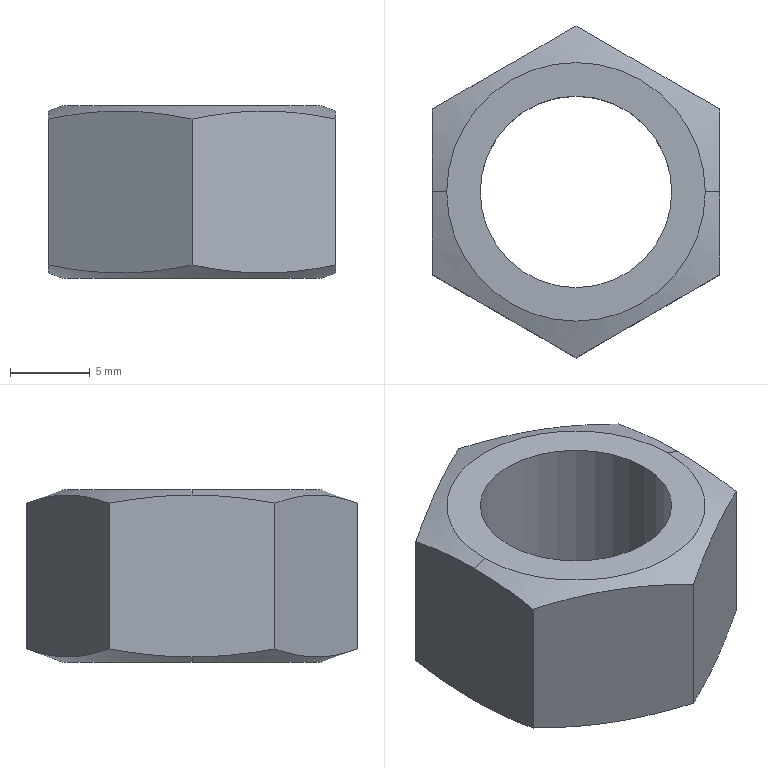Part | SolidWorks | features Extrusion 1, ICE 1, MirrorPattern 1, RefAxis 1, RevCut 1 | 1 solid | 14 faces | box 18 x 20.785 x 10.8 mm | volume 1768 mm3 | plane 8 | cone 4 | cylinder 2 | commonest cylinder face diameters 12 x2
STEP:
#1=CARTESIAN_POINT('',(-6.,0.,0.));
#2=VERTEX_POINT('',#1);
#3=CARTESIAN_POINT('',(6.,0.,0.));
#4=VERTEX_POINT('',#3);
#5=CARTESIAN_POINT('',(0.,0.,0.));
#6=DIRECTION('',(0.,0.,1.));
#7=DIRECTION('',(1.,0.,0.));
#8=AXIS2_PLACEMENT_3D('',#5,#6,#7);
#9=CIRCLE('',#8,6.);
#10=EDGE_CURVE('',#2,#4,#9,.T.);
#11=ORIENTED_EDGE('',*,*,#10,.F.);
#12=CARTESIAN_POINT('',(-6.,0.,10.8));
#13=VERTEX_POINT('',#12);
#14=CARTESIAN_POINT('',(-6.,0.,0.));
#15=DIRECTION('',(0.,0.,1.));
#16=VECTOR('',#15,1000.);
#17=LINE('',#14,#16);
#18=EDGE_CURVE('',#2,#13,#17,.T.);
#19=ORIENTED_EDGE('',*,*,#18,.T.);
#20=CARTESIAN_POINT('',(6.,0.,10.8));
#21=VERTEX_POINT('',#20);
#22=CARTESIAN_POINT('',(0.,0.,10.8));
#23=DIRECTION('',(0.,0.,1.));
#24=DIRECTION('',(1.,0.,0.));
#25=AXIS2_PLACEMENT_3D('',#22,#23,#24);
#26=CIRCLE('',#25,6.);
#27=EDGE_CURVE('',#13,#21,#26,.T.);
#28=ORIENTED_EDGE('',*,*,#27,.T.);
#29=CARTESIAN_POINT('',(6.,0.,0.));
#30=DIRECTION('',(0.,0.,1.));
#31=VECTOR('',#30,1000.);
#32=LINE('',#29,#31);
#33=EDGE_CURVE('',#4,#21,#32,.T.);
#34=ORIENTED_EDGE('',*,*,#33,.F.);
#35=EDGE_LOOP('',(#11,#19,#28,#34));
#36=FACE_OUTER_BOUND('',#35,.T.);
#37=CARTESIAN_POINT('',(0.,0.,0.));
#38=DIRECTION('',(0.,0.,1.));
#39=DIRECTION('',(1.,0.,0.));
#40=AXIS2_PLACEMENT_3D('',#37,#38,#39);
#41=CYLINDRICAL_SURFACE('',#40,6.);
#42=ADVANCED_FACE('',(#36),#41,.F.);
#43=CARTESIAN_POINT('',(-8.1,0.,0.));
#44=VERTEX_POINT('',#43);
#45=CARTESIAN_POINT('',(8.1,0.,0.));
#46=VERTEX_POINT('',#45);
#47=CARTESIAN_POINT('',(0.,0.,0.));
#48=DIRECTION('',(0.,0.,1.));
#49=DIRECTION('',(1.,0.,0.));
#50=AXIS2_PLACEMENT_3D('',#47,#48,#49);
#51=CIRCLE('',#50,8.1);
#52=EDGE_CURVE('',#44,#46,#51,.T.);
#53=ORIENTED_EDGE('',*,*,#52,.T.);
#54=CARTESIAN_POINT('',(9.,0.,0.3276));
#55=VERTEX_POINT('',#54);
#56=CARTESIAN_POINT('',(10.392,0.,0.8343));
#57=DIRECTION('',(0.9397,0.,0.342));
#58=VECTOR('',#57,1000.);
#59=LINE('',#56,#58);
#60=EDGE_CURVE('',#46,#55,#59,.T.);
#61=ORIENTED_EDGE('',*,*,#60,.T.);
#62=CARTESIAN_POINT('',(9.,-5.196,0.8343));
#63=VERTEX_POINT('',#62);
#64=CARTESIAN_POINT('',(9.,-5.196,0.8343));
#65=CARTESIAN_POINT('',(9.,-4.336,0.6778));
#66=CARTESIAN_POINT('',(9.,-3.466,0.549));
#67=CARTESIAN_POINT('',(9.,-1.732,0.3738));
#68=CARTESIAN_POINT('',(9.,-0.8653,0.3276));
#69=CARTESIAN_POINT('',(9.,0.,0.3276));
#70=B_SPLINE_CURVE_WITH_KNOTS('',3,(#64,#65,#66,#67,#68,#69),.UNSPECIFIED.,.F.,.F.,(4,2,4),(0.008807,0.01143,0.01404),.UNSPECIFIED.);
#71=EDGE_CURVE('',#63,#55,#70,.T.);
#72=ORIENTED_EDGE('',*,*,#71,.F.);
#73=CARTESIAN_POINT('',(0.,-10.392,0.8343));
#74=VERTEX_POINT('',#73);
#75=CARTESIAN_POINT('',(0.,-10.392,0.8343));
#76=CARTESIAN_POINT('',(0.75,-9.959,0.6767));
#77=CARTESIAN_POINT('',(1.5,-9.526,0.5488));
#78=CARTESIAN_POINT('',(3.,-8.66,0.3739));
#79=CARTESIAN_POINT('',(4.5,-7.794,0.2812));
#80=CARTESIAN_POINT('',(6.,-6.928,0.3739));
#81=CARTESIAN_POINT('',(7.5,-6.062,0.5488));
#82=CARTESIAN_POINT('',(8.25,-5.629,0.6767));
#83=CARTESIAN_POINT('',(9.,-5.196,0.8343));
#84=B_SPLINE_CURVE_WITH_KNOTS('',3,(#75,#76,#77,#78,#79,#80,#81,#82,#83),.UNSPECIFIED.,.F.,.F.,(4,2,1,2,4),(0.000000231,0.002598,0.005196,0.007794,0.01039),.UNSPECIFIED.);
#85=EDGE_CURVE('',#74,#63,#84,.T.);
#86=ORIENTED_EDGE('',*,*,#85,.F.);
#87=CARTESIAN_POINT('',(-9.,-5.196,0.8343));
#88=VERTEX_POINT('',#87);
#89=CARTESIAN_POINT('',(-9.,-5.196,0.8343));
#90=CARTESIAN_POINT('',(-8.25,-5.629,0.6767));
#91=CARTESIAN_POINT('',(-7.5,-6.062,0.5488));
#92=CARTESIAN_POINT('',(-6.,-6.928,0.3739));
#93=CARTESIAN_POINT('',(-4.5,-7.794,0.2812));
#94=CARTESIAN_POINT('',(-3.,-8.66,0.3739));
#95=CARTESIAN_POINT('',(-1.5,-9.526,0.5488));
#96=CARTESIAN_POINT('',(-0.75,-9.959,0.6767));
#97=CARTESIAN_POINT('',(0.,-10.392,0.8343));
#98=B_SPLINE_CURVE_WITH_KNOTS('',3,(#89,#90,#91,#92,#93,#94,#95,#96,#97),.UNSPECIFIED.,.F.,.F.,(4,2,1,2,4),(0.000000231,0.002598,0.005196,0.007794,0.01039),.UNSPECIFIED.);
#99=EDGE_CURVE('',#88,#74,#98,.T.);
#100=ORIENTED_EDGE('',*,*,#99,.F.);
#101=CARTESIAN_POINT('',(-9.,0.,0.3276));
#102=VERTEX_POINT('',#101);
#103=CARTESIAN_POINT('',(-9.,0.,0.3276));
#104=CARTESIAN_POINT('',(-9.,-0.8653,0.3276));
#105=CARTESIAN_POINT('',(-9.,-1.732,0.3738));
#106=CARTESIAN_POINT('',(-9.,-3.466,0.549));
#107=CARTESIAN_POINT('',(-9.,-4.336,0.6778));
#108=CARTESIAN_POINT('',(-9.,-5.196,0.8343));
#109=B_SPLINE_CURVE_WITH_KNOTS('',3,(#103,#104,#105,#106,#107,#108),.UNSPECIFIED.,.F.,.F.,(4,2,4),(0.0241,0.02671,0.02932),.UNSPECIFIED.);
#110=EDGE_CURVE('',#102,#88,#109,.T.);
#111=ORIENTED_EDGE('',*,*,#110,.F.);
#112=CARTESIAN_POINT('',(-10.392,0.,0.8343));
#113=DIRECTION('',(-0.9397,0.,0.342));
#114=VECTOR('',#113,1000.);
#115=LINE('',#112,#114);
#116=EDGE_CURVE('',#44,#102,#115,.T.);
#117=ORIENTED_EDGE('',*,*,#116,.F.);
#118=EDGE_LOOP('',(#53,#61,#72,#86,#100,#111,#117));
#119=FACE_OUTER_BOUND('',#118,.T.);
#120=CARTESIAN_POINT('',(0.,0.,0.8343));
#121=DIRECTION('',(0.,0.,1.));
#122=DIRECTION('',(-1.,0.,0.));
#123=AXIS2_PLACEMENT_3D('',#120,#121,#122);
#124=CONICAL_SURFACE('',#123,10.392,1.222);
#125=ADVANCED_FACE('',(#119),#124,.T.);
#126=CARTESIAN_POINT('',(8.1,0.,10.8));
#127=VERTEX_POINT('',#126);
#128=CARTESIAN_POINT('',(-8.1,0.,10.8));
#129=VERTEX_POINT('',#128);
#130=CARTESIAN_POINT('',(0.,0.,10.8));
#131=DIRECTION('',(0.,0.,1.));
#132=DIRECTION('',(1.,0.,0.));
#133=AXIS2_PLACEMENT_3D('',#130,#131,#132);
#134=CIRCLE('',#133,8.1);
#135=EDGE_CURVE('',#127,#129,#134,.T.);
#136=ORIENTED_EDGE('',*,*,#135,.F.);
#137=CARTESIAN_POINT('',(9.,0.,10.472));
#138=VERTEX_POINT('',#137);
#139=CARTESIAN_POINT('',(10.392,0.,9.966));
#140=DIRECTION('',(0.9397,0.,-0.342));
#141=VECTOR('',#140,1000.);
#142=LINE('',#139,#141);
#143=EDGE_CURVE('',#127,#138,#142,.T.);
#144=ORIENTED_EDGE('',*,*,#143,.T.);
#145=CARTESIAN_POINT('',(9.,5.196,9.966));
#146=VERTEX_POINT('',#145);
#147=CARTESIAN_POINT('',(9.,5.196,9.966));
#148=CARTESIAN_POINT('',(9.,4.332,10.123));
#149=CARTESIAN_POINT('',(9.,3.467,10.251));
#150=CARTESIAN_POINT('',(9.,1.735,10.426));
#151=CARTESIAN_POINT('',(9.,0.8679,10.472));
#152=CARTESIAN_POINT('',(9.,0.,10.472));
#153=B_SPLINE_CURVE_WITH_KNOTS('',3,(#147,#148,#149,#150,#151,#152),.UNSPECIFIED.,.F.,.F.,(4,2,4),(0.01886,0.02148,0.0241),.UNSPECIFIED.);
#154=EDGE_CURVE('',#146,#138,#153,.T.);
#155=ORIENTED_EDGE('',*,*,#154,.F.);
#156=CARTESIAN_POINT('',(0.,10.392,9.966));
#157=VERTEX_POINT('',#156);
#158=CARTESIAN_POINT('',(0.,10.392,9.966));
#159=CARTESIAN_POINT('',(0.75,9.959,10.123));
#160=CARTESIAN_POINT('',(1.5,9.526,10.251));
#161=CARTESIAN_POINT('',(3.,8.66,10.426));
#162=CARTESIAN_POINT('',(4.5,7.794,10.519));
#163=CARTESIAN_POINT('',(6.,6.928,10.426));
#164=CARTESIAN_POINT('',(7.5,6.062,10.251));
#165=CARTESIAN_POINT('',(8.25,5.629,10.123));
#166=CARTESIAN_POINT('',(9.,5.196,9.966));
#167=B_SPLINE_CURVE_WITH_KNOTS('',3,(#158,#159,#160,#161,#162,#163,#164,#165,#166),.UNSPECIFIED.,.F.,.F.,(4,2,1,2,4),(0.000000231,0.002598,0.005196,0.007794,0.01039),.UNSPECIFIED.);
#168=EDGE_CURVE('',#157,#146,#167,.T.);
#169=ORIENTED_EDGE('',*,*,#168,.F.);
#170=CARTESIAN_POINT('',(-9.,5.196,9.966));
#171=VERTEX_POINT('',#170);
#172=CARTESIAN_POINT('',(-9.,5.196,9.966));
#173=CARTESIAN_POINT('',(-8.25,5.629,10.123));
#174=CARTESIAN_POINT('',(-7.5,6.062,10.251));
#175=CARTESIAN_POINT('',(-6.,6.928,10.426));
#176=CARTESIAN_POINT('',(-4.5,7.794,10.519));
#177=CARTESIAN_POINT('',(-3.,8.66,10.426));
#178=CARTESIAN_POINT('',(-1.5,9.526,10.251));
#179=CARTESIAN_POINT('',(-0.75,9.959,10.123));
#180=CARTESIAN_POINT('',(0.,10.392,9.966));
#181=B_SPLINE_CURVE_WITH_KNOTS('',3,(#172,#173,#174,#175,#176,#177,#178,#179,#180),.UNSPECIFIED.,.F.,.F.,(4,2,1,2,4),(0.000000231,0.002598,0.005196,0.007794,0.01039),.UNSPECIFIED.);
#182=EDGE_CURVE('',#171,#157,#181,.T.);
#183=ORIENTED_EDGE('',*,*,#182,.F.);
#184=CARTESIAN_POINT('',(-9.,0.,10.472));
#185=VERTEX_POINT('',#184);
#186=CARTESIAN_POINT('',(-9.,0.,10.472));
#187=CARTESIAN_POINT('',(-9.,0.8679,10.472));
#188=CARTESIAN_POINT('',(-9.,1.735,10.426));
#189=CARTESIAN_POINT('',(-9.,3.467,10.251));
#190=CARTESIAN_POINT('',(-9.,4.332,10.123));
#191=CARTESIAN_POINT('',(-9.,5.196,9.966));
#192=B_SPLINE_CURVE_WITH_KNOTS('',3,(#186,#187,#188,#189,#190,#191),.UNSPECIFIED.,.F.,.F.,(4,2,4),(0.01404,0.01667,0.0193),.UNSPECIFIED.);
#193=EDGE_CURVE('',#185,#171,#192,.T.);
#194=ORIENTED_EDGE('',*,*,#193,.F.);
#195=CARTESIAN_POINT('',(-10.392,0.,9.966));
#196=DIRECTION('',(-0.9397,0.,-0.342));
#197=VECTOR('',#196,1000.);
#198=LINE('',#195,#197);
#199=EDGE_CURVE('',#129,#185,#198,.T.);
#200=ORIENTED_EDGE('',*,*,#199,.F.);
#201=EDGE_LOOP('',(#136,#144,#155,#169,#183,#194,#200));
#202=FACE_OUTER_BOUND('',#201,.T.);
#203=CARTESIAN_POINT('',(0.,0.,9.966));
#204=DIRECTION('',(0.,0.,-1.));
#205=DIRECTION('',(-1.,0.,0.));
#206=AXIS2_PLACEMENT_3D('',#203,#204,#205);
#207=CONICAL_SURFACE('',#206,10.392,1.222);
#208=ADVANCED_FACE('',(#202),#207,.T.);
#209=CARTESIAN_POINT('',(9.,5.196,0.8343));
#210=VERTEX_POINT('',#209);
#211=CARTESIAN_POINT('',(9.,5.196,10.8));
#212=DIRECTION('',(0.,0.,-1.));
#213=VECTOR('',#212,1000.);
#214=LINE('',#211,#213);
#215=EDGE_CURVE('',#146,#210,#214,.T.);
#216=ORIENTED_EDGE('',*,*,#215,.T.);
#217=CARTESIAN_POINT('',(0.,10.392,0.8343));
#218=VERTEX_POINT('',#217);
#219=CARTESIAN_POINT('',(9.,5.196,0.8343));
#220=CARTESIAN_POINT('',(8.25,5.629,0.6767));
#221=CARTESIAN_POINT('',(7.5,6.062,0.5488));
#222=CARTESIAN_POINT('',(6.,6.928,0.3739));
#223=CARTESIAN_POINT('',(4.5,7.794,0.2812));
#224=CARTESIAN_POINT('',(3.,8.66,0.3739));
#225=CARTESIAN_POINT('',(1.5,9.526,0.5488));
#226=CARTESIAN_POINT('',(0.75,9.959,0.6767));
#227=CARTESIAN_POINT('',(0.,10.392,0.8343));
#228=B_SPLINE_CURVE_WITH_KNOTS('',3,(#219,#220,#221,#222,#223,#224,#225,#226,#227),.UNSPECIFIED.,.F.,.F.,(4,2,1,2,4),(0.000000231,0.002598,0.005196,0.007794,0.01039),.UNSPECIFIED.);
#229=EDGE_CURVE('',#210,#218,#228,.T.);
#230=ORIENTED_EDGE('',*,*,#229,.T.);
#231=CARTESIAN_POINT('',(0.,10.392,10.8));
#232=DIRECTION('',(0.,0.,-1.));
#233=VECTOR('',#232,1000.);
#234=LINE('',#231,#233);
#235=EDGE_CURVE('',#157,#218,#234,.T.);
#236=ORIENTED_EDGE('',*,*,#235,.F.);
#237=ORIENTED_EDGE('',*,*,#168,.T.);
#238=EDGE_LOOP('',(#216,#230,#236,#237));
#239=FACE_OUTER_BOUND('',#238,.T.);
#240=CARTESIAN_POINT('',(9.,5.196,10.8));
#241=DIRECTION('',(-0.5,-0.866,0.));
#242=DIRECTION('',(0.866,-0.5,0.));
#243=AXIS2_PLACEMENT_3D('',#240,#241,#242);
#244=PLANE('',#243);
#245=ADVANCED_FACE('',(#239),#244,.F.);
#246=ORIENTED_EDGE('',*,*,#235,.T.);
#247=CARTESIAN_POINT('',(-9.,5.196,0.8343));
#248=VERTEX_POINT('',#247);
#249=CARTESIAN_POINT('',(0.,10.392,0.8343));
#250=CARTESIAN_POINT('',(-0.75,9.959,0.6767));
#251=CARTESIAN_POINT('',(-1.5,9.526,0.5488));
#252=CARTESIAN_POINT('',(-3.,8.66,0.3739));
#253=CARTESIAN_POINT('',(-4.5,7.794,0.2812));
#254=CARTESIAN_POINT('',(-6.,6.928,0.3739));
#255=CARTESIAN_POINT('',(-7.5,6.062,0.5488));
#256=CARTESIAN_POINT('',(-8.25,5.629,0.6767));
#257=CARTESIAN_POINT('',(-9.,5.196,0.8343));
#258=B_SPLINE_CURVE_WITH_KNOTS('',3,(#249,#250,#251,#252,#253,#254,#255,#256,#257),.UNSPECIFIED.,.F.,.F.,(4,2,1,2,4),(0.000000231,0.002598,0.005196,0.007794,0.01039),.UNSPECIFIED.);
#259=EDGE_CURVE('',#218,#248,#258,.T.);
#260=ORIENTED_EDGE('',*,*,#259,.T.);
#261=CARTESIAN_POINT('',(-9.,5.196,10.8));
#262=DIRECTION('',(0.,0.,-1.));
#263=VECTOR('',#262,1000.);
#264=LINE('',#261,#263);
#265=EDGE_CURVE('',#171,#248,#264,.T.);
#266=ORIENTED_EDGE('',*,*,#265,.F.);
#267=ORIENTED_EDGE('',*,*,#182,.T.);
#268=EDGE_LOOP('',(#246,#260,#266,#267));
#269=FACE_OUTER_BOUND('',#268,.T.);
#270=CARTESIAN_POINT('',(0.,10.392,10.8));
#271=DIRECTION('',(0.5,-0.866,0.));
#272=DIRECTION('',(0.866,0.5,0.));
#273=AXIS2_PLACEMENT_3D('',#270,#271,#272);
#274=PLANE('',#273);
#275=ADVANCED_FACE('',(#269),#274,.F.);
#276=ORIENTED_EDGE('',*,*,#265,.T.);
#277=CARTESIAN_POINT('',(-9.,5.196,0.8343));
#278=CARTESIAN_POINT('',(-9.,4.332,0.6771));
#279=CARTESIAN_POINT('',(-9.,3.467,0.5491));
#280=CARTESIAN_POINT('',(-9.,1.735,0.3741));
#281=CARTESIAN_POINT('',(-9.,0.8679,0.3276));
#282=CARTESIAN_POINT('',(-9.,0.,0.3276));
#283=B_SPLINE_CURVE_WITH_KNOTS('',3,(#277,#278,#279,#280,#281,#282),.UNSPECIFIED.,.F.,.F.,(4,2,4),(0.01886,0.02148,0.0241),.UNSPECIFIED.);
#284=EDGE_CURVE('',#248,#102,#283,.T.);
#285=ORIENTED_EDGE('',*,*,#284,.T.);
#286=ORIENTED_EDGE('',*,*,#110,.T.);
#287=CARTESIAN_POINT('',(-9.,-5.196,9.966));
#288=VERTEX_POINT('',#287);
#289=CARTESIAN_POINT('',(-9.,-5.196,10.8));
#290=DIRECTION('',(0.,0.,-1.));
#291=VECTOR('',#290,1000.);
#292=LINE('',#289,#291);
#293=EDGE_CURVE('',#288,#88,#292,.T.);
#294=ORIENTED_EDGE('',*,*,#293,.F.);
#295=CARTESIAN_POINT('',(-9.,-5.196,9.966));
#296=CARTESIAN_POINT('',(-9.,-4.336,10.122));
#297=CARTESIAN_POINT('',(-9.,-3.466,10.251));
#298=CARTESIAN_POINT('',(-9.,-1.732,10.426));
#299=CARTESIAN_POINT('',(-9.,-0.8653,10.472));
#300=CARTESIAN_POINT('',(-9.,0.,10.472));
#301=B_SPLINE_CURVE_WITH_KNOTS('',3,(#295,#296,#297,#298,#299,#300),.UNSPECIFIED.,.F.,.F.,(4,2,4),(0.008807,0.01143,0.01404),.UNSPECIFIED.);
#302=EDGE_CURVE('',#288,#185,#301,.T.);
#303=ORIENTED_EDGE('',*,*,#302,.T.);
#304=ORIENTED_EDGE('',*,*,#193,.T.);
#305=EDGE_LOOP('',(#276,#285,#286,#294,#303,#304));
#306=FACE_OUTER_BOUND('',#305,.T.);
#307=CARTESIAN_POINT('',(-9.,5.196,10.8));
#308=DIRECTION('',(1.,0.,0.));
#309=DIRECTION('',(0.,0.,-1.));
#310=AXIS2_PLACEMENT_3D('',#307,#308,#309);
#311=PLANE('',#310);
#312=ADVANCED_FACE('',(#306),#311,.F.);
#313=ORIENTED_EDGE('',*,*,#293,.T.);
#314=ORIENTED_EDGE('',*,*,#99,.T.);
#315=CARTESIAN_POINT('',(0.,-10.392,9.966));
#316=VERTEX_POINT('',#315);
#317=CARTESIAN_POINT('',(0.,-10.392,10.8));
#318=DIRECTION('',(0.,0.,-1.));
#319=VECTOR('',#318,1000.);
#320=LINE('',#317,#319);
#321=EDGE_CURVE('',#316,#74,#320,.T.);
#322=ORIENTED_EDGE('',*,*,#321,.F.);
#323=CARTESIAN_POINT('',(0.,-10.392,9.966));
#324=CARTESIAN_POINT('',(-0.75,-9.959,10.123));
#325=CARTESIAN_POINT('',(-1.5,-9.526,10.251));
#326=CARTESIAN_POINT('',(-3.,-8.66,10.426));
#327=CARTESIAN_POINT('',(-4.5,-7.794,10.519));
#328=CARTESIAN_POINT('',(-6.,-6.928,10.426));
#329=CARTESIAN_POINT('',(-7.5,-6.062,10.251));
#330=CARTESIAN_POINT('',(-8.25,-5.629,10.123));
#331=CARTESIAN_POINT('',(-9.,-5.196,9.966));
#332=B_SPLINE_CURVE_WITH_KNOTS('',3,(#323,#324,#325,#326,#327,#328,#329,#330,#331),.UNSPECIFIED.,.F.,.F.,(4,2,1,2,4),(0.000000231,0.002598,0.005196,0.007794,0.01039),.UNSPECIFIED.);
#333=EDGE_CURVE('',#316,#288,#332,.T.);
#334=ORIENTED_EDGE('',*,*,#333,.T.);
#335=EDGE_LOOP('',(#313,#314,#322,#334));
#336=FACE_OUTER_BOUND('',#335,.T.);
#337=CARTESIAN_POINT('',(-9.,-5.196,10.8));
#338=DIRECTION('',(0.5,0.866,0.));
#339=DIRECTION('',(-0.866,0.5,0.));
#340=AXIS2_PLACEMENT_3D('',#337,#338,#339);
#341=PLANE('',#340);
#342=ADVANCED_FACE('',(#336),#341,.F.);
#343=ORIENTED_EDGE('',*,*,#321,.T.);
#344=ORIENTED_EDGE('',*,*,#85,.T.);
#345=CARTESIAN_POINT('',(9.,-5.196,9.966));
#346=VERTEX_POINT('',#345);
#347=CARTESIAN_POINT('',(9.,-5.196,10.8));
#348=DIRECTION('',(0.,0.,-1.));
#349=VECTOR('',#348,1000.);
#350=LINE('',#347,#349);
#351=EDGE_CURVE('',#346,#63,#350,.T.);
#352=ORIENTED_EDGE('',*,*,#351,.F.);
#353=CARTESIAN_POINT('',(9.,-5.196,9.966));
#354=CARTESIAN_POINT('',(8.25,-5.629,10.123));
#355=CARTESIAN_POINT('',(7.5,-6.062,10.251));
#356=CARTESIAN_POINT('',(6.,-6.928,10.426));
#357=CARTESIAN_POINT('',(4.5,-7.794,10.519));
#358=CARTESIAN_POINT('',(3.,-8.66,10.426));
#359=CARTESIAN_POINT('',(1.5,-9.526,10.251));
#360=CARTESIAN_POINT('',(0.75,-9.959,10.123));
#361=CARTESIAN_POINT('',(0.,-10.392,9.966));
#362=B_SPLINE_CURVE_WITH_KNOTS('',3,(#353,#354,#355,#356,#357,#358,#359,#360,#361),.UNSPECIFIED.,.F.,.F.,(4,2,1,2,4),(0.000000231,0.002598,0.005196,0.007794,0.01039),.UNSPECIFIED.);
#363=EDGE_CURVE('',#346,#316,#362,.T.);
#364=ORIENTED_EDGE('',*,*,#363,.T.);
#365=EDGE_LOOP('',(#343,#344,#352,#364));
#366=FACE_OUTER_BOUND('',#365,.T.);
#367=CARTESIAN_POINT('',(0.,-10.392,10.8));
#368=DIRECTION('',(-0.5,0.866,0.));
#369=DIRECTION('',(-0.866,-0.5,0.));
#370=AXIS2_PLACEMENT_3D('',#367,#368,#369);
#371=PLANE('',#370);
#372=ADVANCED_FACE('',(#366),#371,.F.);
#373=ORIENTED_EDGE('',*,*,#351,.T.);
#374=ORIENTED_EDGE('',*,*,#71,.T.);
#375=CARTESIAN_POINT('',(9.,0.,0.3276));
#376=CARTESIAN_POINT('',(9.,0.8679,0.3276));
#377=CARTESIAN_POINT('',(9.,1.735,0.3741));
#378=CARTESIAN_POINT('',(9.,3.467,0.5491));
#379=CARTESIAN_POINT('',(9.,4.332,0.6771));
#380=CARTESIAN_POINT('',(9.,5.196,0.8343));
#381=B_SPLINE_CURVE_WITH_KNOTS('',3,(#375,#376,#377,#378,#379,#380),.UNSPECIFIED.,.F.,.F.,(4,2,4),(0.01404,0.01667,0.0193),.UNSPECIFIED.);
#382=EDGE_CURVE('',#55,#210,#381,.T.);
#383=ORIENTED_EDGE('',*,*,#382,.T.);
#384=ORIENTED_EDGE('',*,*,#215,.F.);
#385=ORIENTED_EDGE('',*,*,#154,.T.);
#386=CARTESIAN_POINT('',(9.,0.,10.472));
#387=CARTESIAN_POINT('',(9.,-0.8653,10.472));
#388=CARTESIAN_POINT('',(9.,-1.732,10.426));
#389=CARTESIAN_POINT('',(9.,-3.466,10.251));
#390=CARTESIAN_POINT('',(9.,-4.336,10.122));
#391=CARTESIAN_POINT('',(9.,-5.196,9.966));
#392=B_SPLINE_CURVE_WITH_KNOTS('',3,(#386,#387,#388,#389,#390,#391),.UNSPECIFIED.,.F.,.F.,(4,2,4),(0.0241,0.02671,0.02932),.UNSPECIFIED.);
#393=EDGE_CURVE('',#138,#346,#392,.T.);
#394=ORIENTED_EDGE('',*,*,#393,.T.);
#395=EDGE_LOOP('',(#373,#374,#383,#384,#385,#394));
#396=FACE_OUTER_BOUND('',#395,.T.);
#397=CARTESIAN_POINT('',(9.,-5.196,10.8));
#398=DIRECTION('',(-1.,0.,0.));
#399=DIRECTION('',(0.,0.,1.));
#400=AXIS2_PLACEMENT_3D('',#397,#398,#399);
#401=PLANE('',#400);
#402=ADVANCED_FACE('',(#396),#401,.F.);
#403=ORIENTED_EDGE('',*,*,#143,.F.);
#404=CARTESIAN_POINT('',(0.,0.,10.8));
#405=DIRECTION('',(0.,0.,1.));
#406=DIRECTION('',(1.,0.,0.));
#407=AXIS2_PLACEMENT_3D('',#404,#405,#406);
#408=CIRCLE('',#407,8.1);
#409=EDGE_CURVE('',#129,#127,#408,.T.);
#410=ORIENTED_EDGE('',*,*,#409,.F.);
#411=ORIENTED_EDGE('',*,*,#199,.T.);
#412=ORIENTED_EDGE('',*,*,#302,.F.);
#413=ORIENTED_EDGE('',*,*,#333,.F.);
#414=ORIENTED_EDGE('',*,*,#363,.F.);
#415=ORIENTED_EDGE('',*,*,#393,.F.);
#416=EDGE_LOOP('',(#403,#410,#411,#412,#413,#414,#415));
#417=FACE_OUTER_BOUND('',#416,.T.);
#418=CARTESIAN_POINT('',(0.,0.,9.966));
#419=DIRECTION('',(0.,0.,-1.));
#420=DIRECTION('',(-1.,0.,0.));
#421=AXIS2_PLACEMENT_3D('',#418,#419,#420);
#422=CONICAL_SURFACE('',#421,10.392,1.222);
#423=ADVANCED_FACE('',(#417),#422,.T.);
#424=CARTESIAN_POINT('',(0.,0.,10.8));
#425=DIRECTION('',(0.,0.,1.));
#426=DIRECTION('',(1.,0.,0.));
#427=AXIS2_PLACEMENT_3D('',#424,#425,#426);
#428=CIRCLE('',#427,6.);
#429=EDGE_CURVE('',#21,#13,#428,.T.);
#430=ORIENTED_EDGE('',*,*,#429,.F.);
#431=ORIENTED_EDGE('',*,*,#27,.F.);
#432=EDGE_LOOP('',(#430,#431));
#433=FACE_BOUND('',#432,.T.);
#434=ORIENTED_EDGE('',*,*,#409,.T.);
#435=ORIENTED_EDGE('',*,*,#135,.T.);
#436=EDGE_LOOP('',(#434,#435));
#437=FACE_OUTER_BOUND('',#436,.T.);
#438=CARTESIAN_POINT('',(0.,0.,10.8));
#439=DIRECTION('',(0.,0.,1.));
#440=DIRECTION('',(1.,0.,0.));
#441=AXIS2_PLACEMENT_3D('',#438,#439,#440);
#442=PLANE('',#441);
#443=ADVANCED_FACE('',(#433,#437),#442,.T.);
#444=ORIENTED_EDGE('',*,*,#60,.F.);
#445=CARTESIAN_POINT('',(0.,0.,0.));
#446=DIRECTION('',(0.,0.,1.));
#447=DIRECTION('',(1.,0.,0.));
#448=AXIS2_PLACEMENT_3D('',#445,#446,#447);
#449=CIRCLE('',#448,8.1);
#450=EDGE_CURVE('',#46,#44,#449,.T.);
#451=ORIENTED_EDGE('',*,*,#450,.T.);
#452=ORIENTED_EDGE('',*,*,#116,.T.);
#453=ORIENTED_EDGE('',*,*,#284,.F.);
#454=ORIENTED_EDGE('',*,*,#259,.F.);
#455=ORIENTED_EDGE('',*,*,#229,.F.);
#456=ORIENTED_EDGE('',*,*,#382,.F.);
#457=EDGE_LOOP('',(#444,#451,#452,#453,#454,#455,#456));
#458=FACE_OUTER_BOUND('',#457,.T.);
#459=CARTESIAN_POINT('',(0.,0.,0.8343));
#460=DIRECTION('',(0.,0.,1.));
#461=DIRECTION('',(-1.,0.,0.));
#462=AXIS2_PLACEMENT_3D('',#459,#460,#461);
#463=CONICAL_SURFACE('',#462,10.392,1.222);
#464=ADVANCED_FACE('',(#458),#463,.T.);
#465=CARTESIAN_POINT('',(0.,0.,0.));
#466=DIRECTION('',(0.,0.,1.));
#467=DIRECTION('',(1.,0.,0.));
#468=AXIS2_PLACEMENT_3D('',#465,#466,#467);
#469=CIRCLE('',#468,6.);
#470=EDGE_CURVE('',#4,#2,#469,.T.);
#471=ORIENTED_EDGE('',*,*,#470,.T.);
#472=ORIENTED_EDGE('',*,*,#10,.T.);
#473=EDGE_LOOP('',(#471,#472));
#474=FACE_BOUND('',#473,.T.);
#475=ORIENTED_EDGE('',*,*,#52,.F.);
#476=ORIENTED_EDGE('',*,*,#450,.F.);
#477=EDGE_LOOP('',(#475,#476));
#478=FACE_OUTER_BOUND('',#477,.T.);
#479=CARTESIAN_POINT('',(0.,0.,0.));
#480=DIRECTION('',(0.,0.,1.));
#481=DIRECTION('',(1.,0.,0.));
#482=AXIS2_PLACEMENT_3D('',#479,#480,#481);
#483=PLANE('',#482);
#484=ADVANCED_FACE('',(#474,#478),#483,.F.);
#485=ORIENTED_EDGE('',*,*,#18,.F.);
#486=ORIENTED_EDGE('',*,*,#470,.F.);
#487=ORIENTED_EDGE('',*,*,#33,.T.);
#488=ORIENTED_EDGE('',*,*,#429,.T.);
#489=EDGE_LOOP('',(#485,#486,#487,#488));
#490=FACE_OUTER_BOUND('',#489,.T.);
#491=CARTESIAN_POINT('',(0.,0.,0.));
#492=DIRECTION('',(0.,0.,1.));
#493=DIRECTION('',(1.,0.,0.));
#494=AXIS2_PLACEMENT_3D('',#491,#492,#493);
#495=CYLINDRICAL_SURFACE('',#494,6.);
#496=ADVANCED_FACE('',(#490),#495,.F.);
#497=CLOSED_SHELL('',(#42,#125,#208,#245,#275,#312,#342,#372,#402,#423,#443,#464,#484,#496));
#498=MANIFOLD_SOLID_BREP('',#497);
#499=CARTESIAN_POINT('',(0.,0.,0.));
#500=DIRECTION('',(0.,0.,1.));
#501=DIRECTION('',(1.,0.,0.));
#502=AXIS2_PLACEMENT_3D('',#499,#500,#501);
#503=(LENGTH_UNIT()NAMED_UNIT(*)SI_UNIT(.MILLI.,.METRE.));
#504=UNCERTAINTY_MEASURE_WITH_UNIT(LENGTH_MEASURE(0.00001),#503,'','');
#505=(NAMED_UNIT(*)PLANE_ANGLE_UNIT()SI_UNIT($,.RADIAN.));
#506=(NAMED_UNIT(*)SI_UNIT($,.STERADIAN.)SOLID_ANGLE_UNIT());
#507=(GEOMETRIC_REPRESENTATION_CONTEXT(3)GLOBAL_UNCERTAINTY_ASSIGNED_CONTEXT((#504))GLOBAL_UNIT_ASSIGNED_CONTEXT((#503,#505,#506))REPRESENTATION_CONTEXT('',''));
#508=ADVANCED_BREP_SHAPE_REPRESENTATION('',(#498,#502),#507);